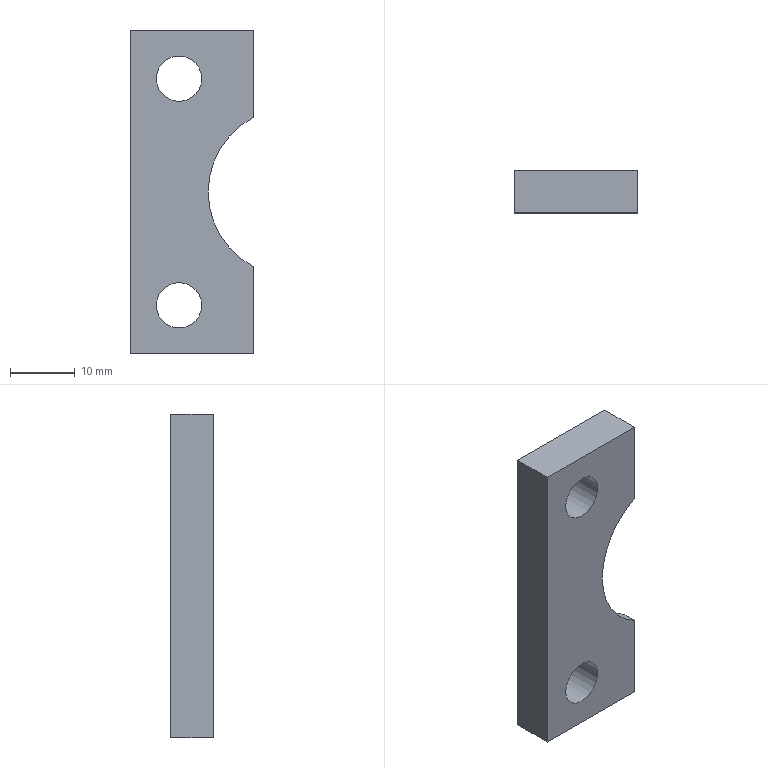Part | NX | features solid 2 | 1 solid | 12 faces | box 19 x 6.5 x 50 mm | volume 4503 mm3 | plane 8 | cylinder 4 | commonest cylinder face diameters 7 x2 26 x1 32 x1
STEP:
#1=CARTESIAN_POINT('',(-706.,844.75,-170.168));
#2=VERTEX_POINT('',#1);
#3=CARTESIAN_POINT('',(-706.,849.,-170.168));
#4=VERTEX_POINT('',#3);
#5=CARTESIAN_POINT('',(-706.,842.5,-170.168));
#6=DIRECTION('',(0.,1.,0.));
#7=VECTOR('',#6,1000.);
#8=LINE('',#5,#7);
#9=EDGE_CURVE('',#2,#4,#8,.T.);
#10=ORIENTED_EDGE('',*,*,#9,.F.);
#11=CARTESIAN_POINT('',(-706.,844.75,-199.832));
#12=VERTEX_POINT('',#11);
#13=CARTESIAN_POINT('',(-700.,844.75,-185.));
#14=DIRECTION('',(0.,-1.,0.));
#15=DIRECTION('',(1.,0.,0.));
#16=AXIS2_PLACEMENT_3D('',#13,#14,#15);
#17=CIRCLE('',#16,16.);
#18=EDGE_CURVE('',#2,#12,#17,.T.);
#19=ORIENTED_EDGE('',*,*,#18,.T.);
#20=CARTESIAN_POINT('',(-706.,849.,-199.832));
#21=VERTEX_POINT('',#20);
#22=CARTESIAN_POINT('',(-706.,842.5,-199.832));
#23=DIRECTION('',(0.,1.,0.));
#24=VECTOR('',#23,1000.);
#25=LINE('',#22,#24);
#26=EDGE_CURVE('',#12,#21,#25,.T.);
#27=ORIENTED_EDGE('',*,*,#26,.T.);
#28=CARTESIAN_POINT('',(-700.,849.,-185.));
#29=DIRECTION('',(0.,-1.,0.));
#30=DIRECTION('',(1.,0.,0.));
#31=AXIS2_PLACEMENT_3D('',#28,#29,#30);
#32=CIRCLE('',#31,16.);
#33=EDGE_CURVE('',#4,#21,#32,.T.);
#34=ORIENTED_EDGE('',*,*,#33,.F.);
#35=EDGE_LOOP('',(#10,#19,#27,#34));
#36=FACE_BOUND('',#35,.T.);
#37=CARTESIAN_POINT('',(-700.,842.5,-185.));
#38=DIRECTION('',(0.,1.,0.));
#39=DIRECTION('',(-1.,0.,0.));
#40=AXIS2_PLACEMENT_3D('',#37,#38,#39);
#41=CYLINDRICAL_SURFACE('',#40,16.);
#42=ADVANCED_FACE('',(#36),#41,.F.);
#43=CARTESIAN_POINT('',(-714.,842.5,-167.5));
#44=VERTEX_POINT('',#43);
#45=CARTESIAN_POINT('',(-717.5,842.5,-167.5));
#46=DIRECTION('',(0.,-1.,0.));
#47=DIRECTION('',(1.,0.,0.));
#48=AXIS2_PLACEMENT_3D('',#45,#46,#47);
#49=CIRCLE('',#48,3.5);
#50=EDGE_CURVE('',#44,#44,#49,.T.);
#51=ORIENTED_EDGE('',*,*,#50,.F.);
#52=EDGE_LOOP('',(#51));
#53=FACE_BOUND('',#52,.T.);
#54=CARTESIAN_POINT('',(-725.,842.5,-160.));
#55=VERTEX_POINT('',#54);
#56=CARTESIAN_POINT('',(-706.,842.5,-160.));
#57=VERTEX_POINT('',#56);
#58=CARTESIAN_POINT('',(-725.,842.5,-160.));
#59=DIRECTION('',(1.,0.,0.));
#60=VECTOR('',#59,1000.);
#61=LINE('',#58,#60);
#62=EDGE_CURVE('',#55,#57,#61,.T.);
#63=ORIENTED_EDGE('',*,*,#62,.F.);
#64=CARTESIAN_POINT('',(-725.,842.5,-210.));
#65=VERTEX_POINT('',#64);
#66=CARTESIAN_POINT('',(-725.,842.5,-210.));
#67=DIRECTION('',(0.,0.,1.));
#68=VECTOR('',#67,1000.);
#69=LINE('',#66,#68);
#70=EDGE_CURVE('',#65,#55,#69,.T.);
#71=ORIENTED_EDGE('',*,*,#70,.F.);
#72=CARTESIAN_POINT('',(-706.,842.5,-210.));
#73=VERTEX_POINT('',#72);
#74=CARTESIAN_POINT('',(-725.,842.5,-210.));
#75=DIRECTION('',(1.,0.,0.));
#76=VECTOR('',#75,1000.);
#77=LINE('',#74,#76);
#78=EDGE_CURVE('',#65,#73,#77,.T.);
#79=ORIENTED_EDGE('',*,*,#78,.T.);
#80=CARTESIAN_POINT('',(-706.,842.5,-196.533));
#81=VERTEX_POINT('',#80);
#82=CARTESIAN_POINT('',(-706.,842.5,-196.533));
#83=DIRECTION('',(0.,0.,-1.));
#84=VECTOR('',#83,1000.);
#85=LINE('',#82,#84);
#86=EDGE_CURVE('',#81,#73,#85,.T.);
#87=ORIENTED_EDGE('',*,*,#86,.F.);
#88=CARTESIAN_POINT('',(-706.,842.5,-173.467));
#89=VERTEX_POINT('',#88);
#90=CARTESIAN_POINT('',(-700.,842.5,-185.));
#91=DIRECTION('',(0.,-1.,0.));
#92=DIRECTION('',(1.,0.,0.));
#93=AXIS2_PLACEMENT_3D('',#90,#91,#92);
#94=CIRCLE('',#93,13.);
#95=EDGE_CURVE('',#89,#81,#94,.T.);
#96=ORIENTED_EDGE('',*,*,#95,.F.);
#97=CARTESIAN_POINT('',(-706.,842.5,-160.));
#98=DIRECTION('',(0.,0.,-1.));
#99=VECTOR('',#98,1000.);
#100=LINE('',#97,#99);
#101=EDGE_CURVE('',#57,#89,#100,.T.);
#102=ORIENTED_EDGE('',*,*,#101,.F.);
#103=EDGE_LOOP('',(#63,#71,#79,#87,#96,#102));
#104=FACE_BOUND('',#103,.T.);
#105=CARTESIAN_POINT('',(-714.,842.5,-202.5));
#106=VERTEX_POINT('',#105);
#107=CARTESIAN_POINT('',(-717.5,842.5,-202.5));
#108=DIRECTION('',(0.,-1.,0.));
#109=DIRECTION('',(1.,0.,0.));
#110=AXIS2_PLACEMENT_3D('',#107,#108,#109);
#111=CIRCLE('',#110,3.5);
#112=EDGE_CURVE('',#106,#106,#111,.T.);
#113=ORIENTED_EDGE('',*,*,#112,.F.);
#114=EDGE_LOOP('',(#113));
#115=FACE_BOUND('',#114,.T.);
#116=CARTESIAN_POINT('',(-712.333,842.5,-176.117));
#117=DIRECTION('',(0.,-1.,0.));
#118=DIRECTION('',(1.,0.,0.));
#119=AXIS2_PLACEMENT_3D('',#116,#117,#118);
#120=PLANE('',#119);
#121=ADVANCED_FACE('',(#53,#104,#115),#120,.T.);
#122=CARTESIAN_POINT('',(-714.,849.,-167.5));
#123=VERTEX_POINT('',#122);
#124=CARTESIAN_POINT('',(-717.5,849.,-167.5));
#125=DIRECTION('',(0.,-1.,0.));
#126=DIRECTION('',(1.,0.,0.));
#127=AXIS2_PLACEMENT_3D('',#124,#125,#126);
#128=CIRCLE('',#127,3.5);
#129=EDGE_CURVE('',#123,#123,#128,.T.);
#130=ORIENTED_EDGE('',*,*,#129,.T.);
#131=EDGE_LOOP('',(#130));
#132=FACE_BOUND('',#131,.T.);
#133=CARTESIAN_POINT('',(-725.,849.,-160.));
#134=VERTEX_POINT('',#133);
#135=CARTESIAN_POINT('',(-706.,849.,-160.));
#136=VERTEX_POINT('',#135);
#137=CARTESIAN_POINT('',(-725.,849.,-160.));
#138=DIRECTION('',(1.,0.,0.));
#139=VECTOR('',#138,1000.);
#140=LINE('',#137,#139);
#141=EDGE_CURVE('',#134,#136,#140,.T.);
#142=ORIENTED_EDGE('',*,*,#141,.T.);
#143=CARTESIAN_POINT('',(-706.,849.,-160.));
#144=DIRECTION('',(0.,0.,-1.));
#145=VECTOR('',#144,1000.);
#146=LINE('',#143,#145);
#147=EDGE_CURVE('',#136,#4,#146,.T.);
#148=ORIENTED_EDGE('',*,*,#147,.T.);
#149=ORIENTED_EDGE('',*,*,#33,.T.);
#150=CARTESIAN_POINT('',(-706.,849.,-210.));
#151=VERTEX_POINT('',#150);
#152=CARTESIAN_POINT('',(-706.,849.,-196.533));
#153=DIRECTION('',(0.,0.,-1.));
#154=VECTOR('',#153,1000.);
#155=LINE('',#152,#154);
#156=EDGE_CURVE('',#21,#151,#155,.T.);
#157=ORIENTED_EDGE('',*,*,#156,.T.);
#158=CARTESIAN_POINT('',(-725.,849.,-210.));
#159=VERTEX_POINT('',#158);
#160=CARTESIAN_POINT('',(-725.,849.,-210.));
#161=DIRECTION('',(1.,0.,0.));
#162=VECTOR('',#161,1000.);
#163=LINE('',#160,#162);
#164=EDGE_CURVE('',#159,#151,#163,.T.);
#165=ORIENTED_EDGE('',*,*,#164,.F.);
#166=CARTESIAN_POINT('',(-725.,849.,-210.));
#167=DIRECTION('',(0.,0.,1.));
#168=VECTOR('',#167,1000.);
#169=LINE('',#166,#168);
#170=EDGE_CURVE('',#159,#134,#169,.T.);
#171=ORIENTED_EDGE('',*,*,#170,.T.);
#172=EDGE_LOOP('',(#142,#148,#149,#157,#165,#171));
#173=FACE_BOUND('',#172,.T.);
#174=CARTESIAN_POINT('',(-714.,849.,-202.5));
#175=VERTEX_POINT('',#174);
#176=CARTESIAN_POINT('',(-717.5,849.,-202.5));
#177=DIRECTION('',(0.,-1.,0.));
#178=DIRECTION('',(1.,0.,0.));
#179=AXIS2_PLACEMENT_3D('',#176,#177,#178);
#180=CIRCLE('',#179,3.5);
#181=EDGE_CURVE('',#175,#175,#180,.T.);
#182=ORIENTED_EDGE('',*,*,#181,.T.);
#183=EDGE_LOOP('',(#182));
#184=FACE_BOUND('',#183,.T.);
#185=CARTESIAN_POINT('',(-712.333,849.,-176.117));
#186=DIRECTION('',(0.,-1.,0.));
#187=DIRECTION('',(1.,0.,0.));
#188=AXIS2_PLACEMENT_3D('',#185,#186,#187);
#189=PLANE('',#188);
#190=ADVANCED_FACE('',(#132,#173,#184),#189,.F.);
#191=ORIENTED_EDGE('',*,*,#141,.F.);
#192=CARTESIAN_POINT('',(-725.,842.5,-160.));
#193=DIRECTION('',(0.,1.,0.));
#194=VECTOR('',#193,1000.);
#195=LINE('',#192,#194);
#196=EDGE_CURVE('',#55,#134,#195,.T.);
#197=ORIENTED_EDGE('',*,*,#196,.F.);
#198=ORIENTED_EDGE('',*,*,#62,.T.);
#199=CARTESIAN_POINT('',(-706.,842.5,-160.));
#200=DIRECTION('',(0.,1.,0.));
#201=VECTOR('',#200,1000.);
#202=LINE('',#199,#201);
#203=EDGE_CURVE('',#57,#136,#202,.T.);
#204=ORIENTED_EDGE('',*,*,#203,.T.);
#205=EDGE_LOOP('',(#191,#197,#198,#204));
#206=FACE_BOUND('',#205,.T.);
#207=CARTESIAN_POINT('',(-725.,842.5,-160.));
#208=DIRECTION('',(0.,0.,1.));
#209=DIRECTION('',(0.,-1.,0.));
#210=AXIS2_PLACEMENT_3D('',#207,#208,#209);
#211=PLANE('',#210);
#212=ADVANCED_FACE('',(#206),#211,.T.);
#213=ORIENTED_EDGE('',*,*,#170,.F.);
#214=CARTESIAN_POINT('',(-725.,842.5,-210.));
#215=DIRECTION('',(0.,1.,0.));
#216=VECTOR('',#215,1000.);
#217=LINE('',#214,#216);
#218=EDGE_CURVE('',#65,#159,#217,.T.);
#219=ORIENTED_EDGE('',*,*,#218,.F.);
#220=ORIENTED_EDGE('',*,*,#70,.T.);
#221=ORIENTED_EDGE('',*,*,#196,.T.);
#222=EDGE_LOOP('',(#213,#219,#220,#221));
#223=FACE_BOUND('',#222,.T.);
#224=CARTESIAN_POINT('',(-725.,842.5,-210.));
#225=DIRECTION('',(-1.,0.,0.));
#226=DIRECTION('',(0.,-1.,0.));
#227=AXIS2_PLACEMENT_3D('',#224,#225,#226);
#228=PLANE('',#227);
#229=ADVANCED_FACE('',(#223),#228,.T.);
#230=ORIENTED_EDGE('',*,*,#164,.T.);
#231=CARTESIAN_POINT('',(-706.,842.5,-210.));
#232=DIRECTION('',(0.,1.,0.));
#233=VECTOR('',#232,1000.);
#234=LINE('',#231,#233);
#235=EDGE_CURVE('',#73,#151,#234,.T.);
#236=ORIENTED_EDGE('',*,*,#235,.F.);
#237=ORIENTED_EDGE('',*,*,#78,.F.);
#238=ORIENTED_EDGE('',*,*,#218,.T.);
#239=EDGE_LOOP('',(#230,#236,#237,#238));
#240=FACE_BOUND('',#239,.T.);
#241=CARTESIAN_POINT('',(-725.,842.5,-210.));
#242=DIRECTION('',(0.,0.,1.));
#243=DIRECTION('',(0.,-1.,0.));
#244=AXIS2_PLACEMENT_3D('',#241,#242,#243);
#245=PLANE('',#244);
#246=ADVANCED_FACE('',(#240),#245,.F.);
#247=ORIENTED_EDGE('',*,*,#156,.F.);
#248=ORIENTED_EDGE('',*,*,#26,.F.);
#249=CARTESIAN_POINT('',(-706.,844.75,-196.533));
#250=VERTEX_POINT('',#249);
#251=CARTESIAN_POINT('',(-706.,844.75,-196.533));
#252=DIRECTION('',(0.,0.,-1.));
#253=VECTOR('',#252,1000.);
#254=LINE('',#251,#253);
#255=EDGE_CURVE('',#250,#12,#254,.T.);
#256=ORIENTED_EDGE('',*,*,#255,.F.);
#257=CARTESIAN_POINT('',(-706.,842.5,-196.533));
#258=DIRECTION('',(0.,1.,0.));
#259=VECTOR('',#258,1000.);
#260=LINE('',#257,#259);
#261=EDGE_CURVE('',#81,#250,#260,.T.);
#262=ORIENTED_EDGE('',*,*,#261,.F.);
#263=ORIENTED_EDGE('',*,*,#86,.T.);
#264=ORIENTED_EDGE('',*,*,#235,.T.);
#265=EDGE_LOOP('',(#247,#248,#256,#262,#263,#264));
#266=FACE_BOUND('',#265,.T.);
#267=CARTESIAN_POINT('',(-706.,842.5,-196.533));
#268=DIRECTION('',(1.,0.,0.));
#269=DIRECTION('',(0.,1.,0.));
#270=AXIS2_PLACEMENT_3D('',#267,#268,#269);
#271=PLANE('',#270);
#272=ADVANCED_FACE('',(#266),#271,.T.);
#273=ORIENTED_EDGE('',*,*,#147,.F.);
#274=ORIENTED_EDGE('',*,*,#203,.F.);
#275=ORIENTED_EDGE('',*,*,#101,.T.);
#276=CARTESIAN_POINT('',(-706.,844.75,-173.467));
#277=VERTEX_POINT('',#276);
#278=CARTESIAN_POINT('',(-706.,842.5,-173.467));
#279=DIRECTION('',(0.,1.,0.));
#280=VECTOR('',#279,1000.);
#281=LINE('',#278,#280);
#282=EDGE_CURVE('',#89,#277,#281,.T.);
#283=ORIENTED_EDGE('',*,*,#282,.T.);
#284=CARTESIAN_POINT('',(-706.,844.75,-160.));
#285=DIRECTION('',(0.,0.,-1.));
#286=VECTOR('',#285,1000.);
#287=LINE('',#284,#286);
#288=EDGE_CURVE('',#2,#277,#287,.T.);
#289=ORIENTED_EDGE('',*,*,#288,.F.);
#290=ORIENTED_EDGE('',*,*,#9,.T.);
#291=EDGE_LOOP('',(#273,#274,#275,#283,#289,#290));
#292=FACE_BOUND('',#291,.T.);
#293=CARTESIAN_POINT('',(-706.,842.5,-160.));
#294=DIRECTION('',(1.,0.,0.));
#295=DIRECTION('',(0.,1.,0.));
#296=AXIS2_PLACEMENT_3D('',#293,#294,#295);
#297=PLANE('',#296);
#298=ADVANCED_FACE('',(#292),#297,.T.);
#299=ORIENTED_EDGE('',*,*,#50,.T.);
#300=EDGE_LOOP('',(#299));
#301=FACE_BOUND('',#300,.T.);
#302=ORIENTED_EDGE('',*,*,#129,.F.);
#303=EDGE_LOOP('',(#302));
#304=FACE_BOUND('',#303,.T.);
#305=CARTESIAN_POINT('',(-717.5,842.5,-167.5));
#306=DIRECTION('',(0.,1.,0.));
#307=DIRECTION('',(-1.,0.,0.));
#308=AXIS2_PLACEMENT_3D('',#305,#306,#307);
#309=CYLINDRICAL_SURFACE('',#308,3.5);
#310=ADVANCED_FACE('',(#301,#304),#309,.F.);
#311=ORIENTED_EDGE('',*,*,#112,.T.);
#312=EDGE_LOOP('',(#311));
#313=FACE_BOUND('',#312,.T.);
#314=ORIENTED_EDGE('',*,*,#181,.F.);
#315=EDGE_LOOP('',(#314));
#316=FACE_BOUND('',#315,.T.);
#317=CARTESIAN_POINT('',(-717.5,842.5,-202.5));
#318=DIRECTION('',(0.,1.,0.));
#319=DIRECTION('',(-1.,0.,0.));
#320=AXIS2_PLACEMENT_3D('',#317,#318,#319);
#321=CYLINDRICAL_SURFACE('',#320,3.5);
#322=ADVANCED_FACE('',(#313,#316),#321,.F.);
#323=CARTESIAN_POINT('',(-700.,844.75,-185.));
#324=DIRECTION('',(0.,-1.,0.));
#325=DIRECTION('',(1.,0.,0.));
#326=AXIS2_PLACEMENT_3D('',#323,#324,#325);
#327=CIRCLE('',#326,13.);
#328=EDGE_CURVE('',#277,#250,#327,.T.);
#329=ORIENTED_EDGE('',*,*,#328,.F.);
#330=ORIENTED_EDGE('',*,*,#282,.F.);
#331=ORIENTED_EDGE('',*,*,#95,.T.);
#332=ORIENTED_EDGE('',*,*,#261,.T.);
#333=EDGE_LOOP('',(#329,#330,#331,#332));
#334=FACE_BOUND('',#333,.T.);
#335=CARTESIAN_POINT('',(-700.,842.5,-185.));
#336=DIRECTION('',(0.,1.,0.));
#337=DIRECTION('',(-1.,0.,0.));
#338=AXIS2_PLACEMENT_3D('',#335,#336,#337);
#339=CYLINDRICAL_SURFACE('',#338,13.);
#340=ADVANCED_FACE('',(#334),#339,.F.);
#341=ORIENTED_EDGE('',*,*,#255,.T.);
#342=ORIENTED_EDGE('',*,*,#18,.F.);
#343=ORIENTED_EDGE('',*,*,#288,.T.);
#344=ORIENTED_EDGE('',*,*,#328,.T.);
#345=EDGE_LOOP('',(#341,#342,#343,#344));
#346=FACE_BOUND('',#345,.T.);
#347=CARTESIAN_POINT('',(-706.,844.75,-175.042));
#348=DIRECTION('',(0.,-1.,0.));
#349=DIRECTION('',(1.,0.,0.));
#350=AXIS2_PLACEMENT_3D('',#347,#348,#349);
#351=PLANE('',#350);
#352=ADVANCED_FACE('',(#346),#351,.F.);
#353=CLOSED_SHELL('',(#42,#121,#190,#212,#229,#246,#272,#298,#310,#322,#340,#352));
#354=MANIFOLD_SOLID_BREP('',#353);
#355=(LENGTH_UNIT()NAMED_UNIT(*)SI_UNIT(.MILLI.,.METRE.));
#356=UNCERTAINTY_MEASURE_WITH_UNIT(LENGTH_MEASURE(0.00001),#355,'','');
#357=(NAMED_UNIT(*)PLANE_ANGLE_UNIT()SI_UNIT($,.RADIAN.));
#358=(NAMED_UNIT(*)SI_UNIT($,.STERADIAN.)SOLID_ANGLE_UNIT());
#359=(GEOMETRIC_REPRESENTATION_CONTEXT(3)GLOBAL_UNCERTAINTY_ASSIGNED_CONTEXT((#356))GLOBAL_UNIT_ASSIGNED_CONTEXT((#355,#357,#358))REPRESENTATION_CONTEXT('',''));
#360=ADVANCED_BREP_SHAPE_REPRESENTATION('',(#354),#359);